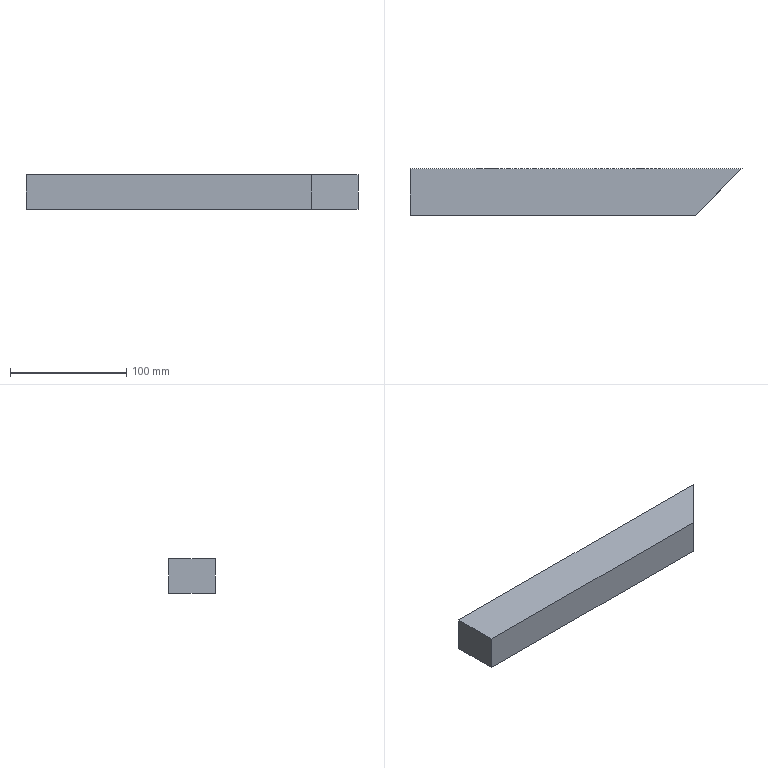Part | SolidWorks | features ICE 3, Extrusion 1 | 1 solid | 12 faces | box 285 x 40 x 30 mm | volume 299150 mm3 | plane 8 | cylinder 4 | commonest cylinder face diameters 20 x4
STEP:
#1=CARTESIAN_POINT('',(-70.,10.,-10.));
#2=VERTEX_POINT('',#1);
#3=CARTESIAN_POINT('',(-70.,10.,10.));
#4=VERTEX_POINT('',#3);
#5=CARTESIAN_POINT('',(-70.,10.,0.));
#6=DIRECTION('',(0.,1.,0.));
#7=DIRECTION('',(0.,0.,-1.));
#8=AXIS2_PLACEMENT_3D('',#5,#6,#7);
#9=CIRCLE('',#8,10.);
#10=EDGE_CURVE('',#2,#4,#9,.T.);
#11=ORIENTED_EDGE('',*,*,#10,.F.);
#12=CARTESIAN_POINT('',(-70.,40.,-10.));
#13=VERTEX_POINT('',#12);
#14=CARTESIAN_POINT('',(-70.,10.,-10.));
#15=DIRECTION('',(0.,1.,0.));
#16=VECTOR('',#15,1000.);
#17=LINE('',#14,#16);
#18=EDGE_CURVE('',#2,#13,#17,.T.);
#19=ORIENTED_EDGE('',*,*,#18,.T.);
#20=CARTESIAN_POINT('',(-70.,40.,10.));
#21=VERTEX_POINT('',#20);
#22=CARTESIAN_POINT('',(-70.,40.,0.));
#23=DIRECTION('',(0.,1.,0.));
#24=DIRECTION('',(0.,0.,-1.));
#25=AXIS2_PLACEMENT_3D('',#22,#23,#24);
#26=CIRCLE('',#25,10.);
#27=EDGE_CURVE('',#13,#21,#26,.T.);
#28=ORIENTED_EDGE('',*,*,#27,.T.);
#29=CARTESIAN_POINT('',(-70.,10.,10.));
#30=DIRECTION('',(0.,1.,0.));
#31=VECTOR('',#30,1000.);
#32=LINE('',#29,#31);
#33=EDGE_CURVE('',#4,#21,#32,.T.);
#34=ORIENTED_EDGE('',*,*,#33,.F.);
#35=EDGE_LOOP('',(#11,#19,#28,#34));
#36=FACE_OUTER_BOUND('',#35,.T.);
#37=CARTESIAN_POINT('',(-70.,10.,0.));
#38=DIRECTION('',(0.,1.,0.));
#39=DIRECTION('',(0.,0.,1.));
#40=AXIS2_PLACEMENT_3D('',#37,#38,#39);
#41=CYLINDRICAL_SURFACE('',#40,10.);
#42=ADVANCED_FACE('',(#36),#41,.F.);
#43=CARTESIAN_POINT('',(70.,10.,-10.));
#44=VERTEX_POINT('',#43);
#45=CARTESIAN_POINT('',(70.,10.,10.));
#46=VERTEX_POINT('',#45);
#47=CARTESIAN_POINT('',(70.,10.,0.));
#48=DIRECTION('',(0.,1.,0.));
#49=DIRECTION('',(0.,0.,1.));
#50=AXIS2_PLACEMENT_3D('',#47,#48,#49);
#51=CIRCLE('',#50,10.);
#52=EDGE_CURVE('',#44,#46,#51,.T.);
#53=ORIENTED_EDGE('',*,*,#52,.F.);
#54=CARTESIAN_POINT('',(70.,40.,-10.));
#55=VERTEX_POINT('',#54);
#56=CARTESIAN_POINT('',(70.,10.,-10.));
#57=DIRECTION('',(0.,1.,0.));
#58=VECTOR('',#57,1000.);
#59=LINE('',#56,#58);
#60=EDGE_CURVE('',#44,#55,#59,.T.);
#61=ORIENTED_EDGE('',*,*,#60,.T.);
#62=CARTESIAN_POINT('',(70.,40.,10.));
#63=VERTEX_POINT('',#62);
#64=CARTESIAN_POINT('',(70.,40.,0.));
#65=DIRECTION('',(0.,1.,0.));
#66=DIRECTION('',(0.,0.,1.));
#67=AXIS2_PLACEMENT_3D('',#64,#65,#66);
#68=CIRCLE('',#67,10.);
#69=EDGE_CURVE('',#55,#63,#68,.T.);
#70=ORIENTED_EDGE('',*,*,#69,.T.);
#71=CARTESIAN_POINT('',(70.,10.,10.));
#72=DIRECTION('',(0.,1.,0.));
#73=VECTOR('',#72,1000.);
#74=LINE('',#71,#73);
#75=EDGE_CURVE('',#46,#63,#74,.T.);
#76=ORIENTED_EDGE('',*,*,#75,.F.);
#77=EDGE_LOOP('',(#53,#61,#70,#76));
#78=FACE_OUTER_BOUND('',#77,.T.);
#79=CARTESIAN_POINT('',(70.,10.,0.));
#80=DIRECTION('',(0.,1.,0.));
#81=DIRECTION('',(0.,0.,1.));
#82=AXIS2_PLACEMENT_3D('',#79,#80,#81);
#83=CYLINDRICAL_SURFACE('',#82,10.);
#84=ADVANCED_FACE('',(#78),#83,.F.);
#85=CARTESIAN_POINT('',(150.,40.,-15.));
#86=VERTEX_POINT('',#85);
#87=CARTESIAN_POINT('',(-135.,40.,-15.));
#88=VERTEX_POINT('',#87);
#89=CARTESIAN_POINT('',(-135.,40.,-15.));
#90=DIRECTION('',(-1.,0.,0.));
#91=VECTOR('',#90,1000.);
#92=LINE('',#89,#91);
#93=EDGE_CURVE('',#86,#88,#92,.T.);
#94=ORIENTED_EDGE('',*,*,#93,.F.);
#95=CARTESIAN_POINT('',(110.,0.,-15.));
#96=VERTEX_POINT('',#95);
#97=CARTESIAN_POINT('',(150.,40.,-15.));
#98=DIRECTION('',(-0.7071,-0.7071,0.));
#99=VECTOR('',#98,1000.);
#100=LINE('',#97,#99);
#101=EDGE_CURVE('',#86,#96,#100,.T.);
#102=ORIENTED_EDGE('',*,*,#101,.T.);
#103=CARTESIAN_POINT('',(-135.,0.,-15.));
#104=VERTEX_POINT('',#103);
#105=CARTESIAN_POINT('',(-135.,0.,-15.));
#106=DIRECTION('',(-1.,0.,0.));
#107=VECTOR('',#106,1000.);
#108=LINE('',#105,#107);
#109=EDGE_CURVE('',#96,#104,#108,.T.);
#110=ORIENTED_EDGE('',*,*,#109,.T.);
#111=CARTESIAN_POINT('',(-135.,40.,-15.));
#112=DIRECTION('',(0.,-1.,0.));
#113=VECTOR('',#112,1000.);
#114=LINE('',#111,#113);
#115=EDGE_CURVE('',#88,#104,#114,.T.);
#116=ORIENTED_EDGE('',*,*,#115,.F.);
#117=EDGE_LOOP('',(#94,#102,#110,#116));
#118=FACE_OUTER_BOUND('',#117,.T.);
#119=CARTESIAN_POINT('',(-135.,40.,-15.));
#120=DIRECTION('',(0.,0.,1.));
#121=DIRECTION('',(1.,0.,0.));
#122=AXIS2_PLACEMENT_3D('',#119,#120,#121);
#123=PLANE('',#122);
#124=ADVANCED_FACE('',(#118),#123,.F.);
#125=CARTESIAN_POINT('',(-135.,0.,15.));
#126=VERTEX_POINT('',#125);
#127=CARTESIAN_POINT('',(-135.,0.,15.));
#128=DIRECTION('',(0.,0.,1.));
#129=VECTOR('',#128,1000.);
#130=LINE('',#127,#129);
#131=EDGE_CURVE('',#104,#126,#130,.T.);
#132=ORIENTED_EDGE('',*,*,#131,.T.);
#133=CARTESIAN_POINT('',(-135.,40.,15.));
#134=VERTEX_POINT('',#133);
#135=CARTESIAN_POINT('',(-135.,40.,15.));
#136=DIRECTION('',(0.,-1.,0.));
#137=VECTOR('',#136,1000.);
#138=LINE('',#135,#137);
#139=EDGE_CURVE('',#134,#126,#138,.T.);
#140=ORIENTED_EDGE('',*,*,#139,.F.);
#141=CARTESIAN_POINT('',(-135.,40.,15.));
#142=DIRECTION('',(0.,0.,1.));
#143=VECTOR('',#142,1000.);
#144=LINE('',#141,#143);
#145=EDGE_CURVE('',#88,#134,#144,.T.);
#146=ORIENTED_EDGE('',*,*,#145,.F.);
#147=ORIENTED_EDGE('',*,*,#115,.T.);
#148=EDGE_LOOP('',(#132,#140,#146,#147));
#149=FACE_OUTER_BOUND('',#148,.T.);
#150=CARTESIAN_POINT('',(-135.,40.,15.));
#151=DIRECTION('',(1.,0.,0.));
#152=DIRECTION('',(0.,0.,-1.));
#153=AXIS2_PLACEMENT_3D('',#150,#151,#152);
#154=PLANE('',#153);
#155=ADVANCED_FACE('',(#149),#154,.F.);
#156=CARTESIAN_POINT('',(110.,0.,15.));
#157=VERTEX_POINT('',#156);
#158=CARTESIAN_POINT('',(-135.,0.,15.));
#159=DIRECTION('',(1.,0.,0.));
#160=VECTOR('',#159,1000.);
#161=LINE('',#158,#160);
#162=EDGE_CURVE('',#126,#157,#161,.T.);
#163=ORIENTED_EDGE('',*,*,#162,.T.);
#164=CARTESIAN_POINT('',(150.,40.,15.));
#165=VERTEX_POINT('',#164);
#166=CARTESIAN_POINT('',(150.,40.,15.));
#167=DIRECTION('',(-0.7071,-0.7071,0.));
#168=VECTOR('',#167,1000.);
#169=LINE('',#166,#168);
#170=EDGE_CURVE('',#165,#157,#169,.T.);
#171=ORIENTED_EDGE('',*,*,#170,.F.);
#172=CARTESIAN_POINT('',(-135.,40.,15.));
#173=DIRECTION('',(1.,0.,0.));
#174=VECTOR('',#173,1000.);
#175=LINE('',#172,#174);
#176=EDGE_CURVE('',#134,#165,#175,.T.);
#177=ORIENTED_EDGE('',*,*,#176,.F.);
#178=ORIENTED_EDGE('',*,*,#139,.T.);
#179=EDGE_LOOP('',(#163,#171,#177,#178));
#180=FACE_OUTER_BOUND('',#179,.T.);
#181=CARTESIAN_POINT('',(-135.,40.,15.));
#182=DIRECTION('',(0.,0.,-1.));
#183=DIRECTION('',(-1.,0.,0.));
#184=AXIS2_PLACEMENT_3D('',#181,#182,#183);
#185=PLANE('',#184);
#186=ADVANCED_FACE('',(#180),#185,.F.);
#187=CARTESIAN_POINT('',(-70.,40.,0.));
#188=DIRECTION('',(0.,1.,0.));
#189=DIRECTION('',(0.,0.,-1.));
#190=AXIS2_PLACEMENT_3D('',#187,#188,#189);
#191=CIRCLE('',#190,10.);
#192=EDGE_CURVE('',#21,#13,#191,.T.);
#193=ORIENTED_EDGE('',*,*,#192,.F.);
#194=ORIENTED_EDGE('',*,*,#27,.F.);
#195=EDGE_LOOP('',(#193,#194));
#196=FACE_BOUND('',#195,.T.);
#197=CARTESIAN_POINT('',(70.,40.,0.));
#198=DIRECTION('',(0.,1.,0.));
#199=DIRECTION('',(0.,0.,1.));
#200=AXIS2_PLACEMENT_3D('',#197,#198,#199);
#201=CIRCLE('',#200,10.);
#202=EDGE_CURVE('',#63,#55,#201,.T.);
#203=ORIENTED_EDGE('',*,*,#202,.F.);
#204=ORIENTED_EDGE('',*,*,#69,.F.);
#205=EDGE_LOOP('',(#203,#204));
#206=FACE_BOUND('',#205,.T.);
#207=ORIENTED_EDGE('',*,*,#176,.T.);
#208=CARTESIAN_POINT('',(150.,40.,-15.));
#209=DIRECTION('',(0.,0.,1.));
#210=VECTOR('',#209,1000.);
#211=LINE('',#208,#210);
#212=EDGE_CURVE('',#86,#165,#211,.T.);
#213=ORIENTED_EDGE('',*,*,#212,.F.);
#214=ORIENTED_EDGE('',*,*,#93,.T.);
#215=ORIENTED_EDGE('',*,*,#145,.T.);
#216=EDGE_LOOP('',(#207,#213,#214,#215));
#217=FACE_OUTER_BOUND('',#216,.T.);
#218=CARTESIAN_POINT('',(0.,40.,0.));
#219=DIRECTION('',(0.,-1.,0.));
#220=DIRECTION('',(0.,0.,-1.));
#221=AXIS2_PLACEMENT_3D('',#218,#219,#220);
#222=PLANE('',#221);
#223=ADVANCED_FACE('',(#196,#206,#217),#222,.F.);
#224=CARTESIAN_POINT('',(110.,0.,-15.));
#225=DIRECTION('',(0.,0.,1.));
#226=VECTOR('',#225,1000.);
#227=LINE('',#224,#226);
#228=EDGE_CURVE('',#96,#157,#227,.T.);
#229=ORIENTED_EDGE('',*,*,#228,.T.);
#230=ORIENTED_EDGE('',*,*,#162,.F.);
#231=ORIENTED_EDGE('',*,*,#131,.F.);
#232=ORIENTED_EDGE('',*,*,#109,.F.);
#233=EDGE_LOOP('',(#229,#230,#231,#232));
#234=FACE_OUTER_BOUND('',#233,.T.);
#235=CARTESIAN_POINT('',(0.,0.,0.));
#236=DIRECTION('',(0.,-1.,0.));
#237=DIRECTION('',(0.,0.,-1.));
#238=AXIS2_PLACEMENT_3D('',#235,#236,#237);
#239=PLANE('',#238);
#240=ADVANCED_FACE('',(#234),#239,.T.);
#241=ORIENTED_EDGE('',*,*,#60,.F.);
#242=CARTESIAN_POINT('',(70.,10.,0.));
#243=DIRECTION('',(0.,1.,0.));
#244=DIRECTION('',(0.,0.,1.));
#245=AXIS2_PLACEMENT_3D('',#242,#243,#244);
#246=CIRCLE('',#245,10.);
#247=EDGE_CURVE('',#46,#44,#246,.T.);
#248=ORIENTED_EDGE('',*,*,#247,.F.);
#249=ORIENTED_EDGE('',*,*,#75,.T.);
#250=ORIENTED_EDGE('',*,*,#202,.T.);
#251=EDGE_LOOP('',(#241,#248,#249,#250));
#252=FACE_OUTER_BOUND('',#251,.T.);
#253=CARTESIAN_POINT('',(70.,10.,0.));
#254=DIRECTION('',(0.,1.,0.));
#255=DIRECTION('',(0.,0.,1.));
#256=AXIS2_PLACEMENT_3D('',#253,#254,#255);
#257=CYLINDRICAL_SURFACE('',#256,10.);
#258=ADVANCED_FACE('',(#252),#257,.F.);
#259=ORIENTED_EDGE('',*,*,#247,.T.);
#260=ORIENTED_EDGE('',*,*,#52,.T.);
#261=EDGE_LOOP('',(#259,#260));
#262=FACE_OUTER_BOUND('',#261,.T.);
#263=CARTESIAN_POINT('',(70.,10.,0.));
#264=DIRECTION('',(0.,1.,0.));
#265=DIRECTION('',(0.,0.,1.));
#266=AXIS2_PLACEMENT_3D('',#263,#264,#265);
#267=PLANE('',#266);
#268=ADVANCED_FACE('',(#262),#267,.T.);
#269=ORIENTED_EDGE('',*,*,#18,.F.);
#270=CARTESIAN_POINT('',(-70.,10.,0.));
#271=DIRECTION('',(0.,1.,0.));
#272=DIRECTION('',(0.,0.,-1.));
#273=AXIS2_PLACEMENT_3D('',#270,#271,#272);
#274=CIRCLE('',#273,10.);
#275=EDGE_CURVE('',#4,#2,#274,.T.);
#276=ORIENTED_EDGE('',*,*,#275,.F.);
#277=ORIENTED_EDGE('',*,*,#33,.T.);
#278=ORIENTED_EDGE('',*,*,#192,.T.);
#279=EDGE_LOOP('',(#269,#276,#277,#278));
#280=FACE_OUTER_BOUND('',#279,.T.);
#281=CARTESIAN_POINT('',(-70.,10.,0.));
#282=DIRECTION('',(0.,1.,0.));
#283=DIRECTION('',(0.,0.,1.));
#284=AXIS2_PLACEMENT_3D('',#281,#282,#283);
#285=CYLINDRICAL_SURFACE('',#284,10.);
#286=ADVANCED_FACE('',(#280),#285,.F.);
#287=ORIENTED_EDGE('',*,*,#275,.T.);
#288=ORIENTED_EDGE('',*,*,#10,.T.);
#289=EDGE_LOOP('',(#287,#288));
#290=FACE_OUTER_BOUND('',#289,.T.);
#291=CARTESIAN_POINT('',(-70.,10.,0.));
#292=DIRECTION('',(0.,-1.,0.));
#293=DIRECTION('',(0.,0.,-1.));
#294=AXIS2_PLACEMENT_3D('',#291,#292,#293);
#295=PLANE('',#294);
#296=ADVANCED_FACE('',(#290),#295,.F.);
#297=ORIENTED_EDGE('',*,*,#170,.T.);
#298=ORIENTED_EDGE('',*,*,#228,.F.);
#299=ORIENTED_EDGE('',*,*,#101,.F.);
#300=ORIENTED_EDGE('',*,*,#212,.T.);
#301=EDGE_LOOP('',(#297,#298,#299,#300));
#302=FACE_OUTER_BOUND('',#301,.T.);
#303=CARTESIAN_POINT('',(150.,40.,-15.));
#304=DIRECTION('',(-0.7071,0.7071,0.));
#305=DIRECTION('',(-0.7071,-0.7071,0.));
#306=AXIS2_PLACEMENT_3D('',#303,#304,#305);
#307=PLANE('',#306);
#308=ADVANCED_FACE('',(#302),#307,.F.);
#309=CLOSED_SHELL('',(#42,#84,#124,#155,#186,#223,#240,#258,#268,#286,#296,#308));
#310=MANIFOLD_SOLID_BREP('',#309);
#311=CARTESIAN_POINT('',(0.,0.,0.));
#312=DIRECTION('',(0.,0.,1.));
#313=DIRECTION('',(1.,0.,0.));
#314=AXIS2_PLACEMENT_3D('',#311,#312,#313);
#315=(LENGTH_UNIT()NAMED_UNIT(*)SI_UNIT(.MILLI.,.METRE.));
#316=UNCERTAINTY_MEASURE_WITH_UNIT(LENGTH_MEASURE(0.00001),#315,'','');
#317=(NAMED_UNIT(*)PLANE_ANGLE_UNIT()SI_UNIT($,.RADIAN.));
#318=(NAMED_UNIT(*)SI_UNIT($,.STERADIAN.)SOLID_ANGLE_UNIT());
#319=(GEOMETRIC_REPRESENTATION_CONTEXT(3)GLOBAL_UNCERTAINTY_ASSIGNED_CONTEXT((#316))GLOBAL_UNIT_ASSIGNED_CONTEXT((#315,#317,#318))REPRESENTATION_CONTEXT('',''));
#320=ADVANCED_BREP_SHAPE_REPRESENTATION('',(#310,#314),#319);